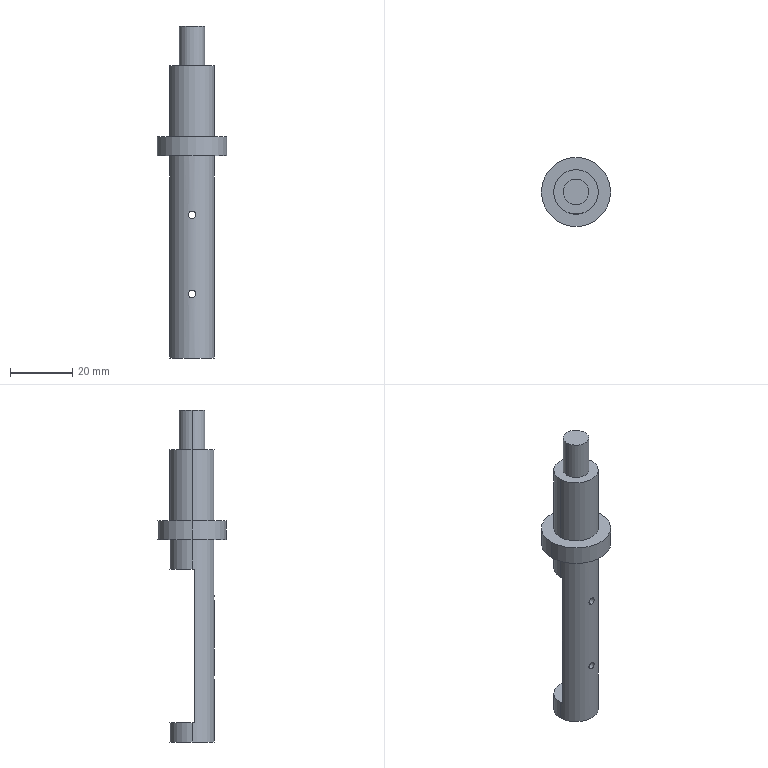Part | SolidWorks | features ICE 6, HoleWzd 2, Extrusion 1, RefAxis 1 | 1 solid | 25 faces | box 22.225 x 22.225 x 106.629 mm | volume 12564 mm3 | cylinder 13 | plane 8 | cone 4 | commonest cylinder face diameters 2.375 x4 14.275 x3 8.255 x2 14.3 x2 22.225 x2
STEP:
#1=CARTESIAN_POINT('',(0.,-0.06425,-2.435));
#2=VERTEX_POINT('',#1);
#3=CARTESIAN_POINT('',(0.,-0.06425,-2.341));
#4=VERTEX_POINT('',#3);
#5=CARTESIAN_POINT('',(0.,-0.06425,-2.388));
#6=DIRECTION('',(0.,1.,0.));
#7=DIRECTION('',(0.,0.,1.));
#8=AXIS2_PLACEMENT_3D('',#5,#6,#7);
#9=CIRCLE('',#8,0.04675);
#10=EDGE_CURVE('',#2,#4,#9,.T.);
#11=ORIENTED_EDGE('',*,*,#10,.F.);
#12=CARTESIAN_POINT('',(0.,-0.03,-2.469));
#13=VERTEX_POINT('',#12);
#14=CARTESIAN_POINT('',(0.,-0.03,-2.469));
#15=DIRECTION('',(0.,0.7071,-0.7071));
#16=VECTOR('',#15,39.37);
#17=LINE('',#14,#16);
#18=EDGE_CURVE('',#2,#13,#17,.T.);
#19=ORIENTED_EDGE('',*,*,#18,.T.);
#20=CARTESIAN_POINT('',(0.,-0.03,-2.307));
#21=VERTEX_POINT('',#20);
#22=CARTESIAN_POINT('',(0.,-0.03,-2.388));
#23=DIRECTION('',(0.,1.,0.));
#24=DIRECTION('',(0.,0.,1.));
#25=AXIS2_PLACEMENT_3D('',#22,#23,#24);
#26=CIRCLE('',#25,0.081);
#27=EDGE_CURVE('',#13,#21,#26,.T.);
#28=ORIENTED_EDGE('',*,*,#27,.T.);
#29=CARTESIAN_POINT('',(0.,-0.03,-2.307));
#30=DIRECTION('',(0.,0.7071,0.7071));
#31=VECTOR('',#30,39.37);
#32=LINE('',#29,#31);
#33=EDGE_CURVE('',#4,#21,#32,.T.);
#34=ORIENTED_EDGE('',*,*,#33,.F.);
#35=EDGE_LOOP('',(#11,#19,#28,#34));
#36=FACE_OUTER_BOUND('',#35,.T.);
#37=CARTESIAN_POINT('',(0.,-0.03,-2.388));
#38=DIRECTION('',(0.,1.,0.));
#39=DIRECTION('',(0.,0.,1.));
#40=AXIS2_PLACEMENT_3D('',#37,#38,#39);
#41=CONICAL_SURFACE('',#40,0.081,0.7854);
#42=ADVANCED_FACE('',(#36),#41,.F.);
#43=CARTESIAN_POINT('',(0.,-0.281,-2.341));
#44=VERTEX_POINT('',#43);
#45=CARTESIAN_POINT('',(0.,-0.281,-2.435));
#46=VERTEX_POINT('',#45);
#47=CARTESIAN_POINT('',(0.,-0.281,-2.341));
#48=CARTESIAN_POINT('',(-0.006189,-0.281,-2.341));
#49=CARTESIAN_POINT('',(-0.01226,-0.2808,-2.342));
#50=CARTESIAN_POINT('',(-0.02358,-0.2801,-2.347));
#51=CARTESIAN_POINT('',(-0.02876,-0.2796,-2.351));
#52=CARTESIAN_POINT('',(-0.03737,-0.2785,-2.359));
#53=CARTESIAN_POINT('',(-0.04085,-0.278,-2.364));
#54=CARTESIAN_POINT('',(-0.04552,-0.2773,-2.376));
#55=CARTESIAN_POINT('',(-0.04675,-0.2771,-2.382));
#56=CARTESIAN_POINT('',(-0.04675,-0.2771,-2.394));
#57=CARTESIAN_POINT('',(-0.04554,-0.2773,-2.4));
#58=CARTESIAN_POINT('',(-0.04084,-0.278,-2.412));
#59=CARTESIAN_POINT('',(-0.03741,-0.2785,-2.417));
#60=CARTESIAN_POINT('',(-0.0287,-0.2796,-2.425));
#61=CARTESIAN_POINT('',(-0.02356,-0.2801,-2.429));
#62=CARTESIAN_POINT('',(-0.01225,-0.2808,-2.434));
#63=CARTESIAN_POINT('',(-0.006108,-0.281,-2.435));
#64=CARTESIAN_POINT('',(0.,-0.281,-2.435));
#65=B_SPLINE_CURVE_WITH_KNOTS('',3,(#47,#48,#49,#50,#51,#52,#53,#54,#55,#56,#57,#58,#59,#60,#61,#62,#63,#64),.UNSPECIFIED.,.F.,.F.,(4,2,2,2,2,2,2,2,4),(0.,0.0004649,0.0009297,0.001395,0.001859,0.002324,0.002789,0.003254,0.003719),.UNSPECIFIED.);
#66=EDGE_CURVE('',#44,#46,#65,.T.);
#67=ORIENTED_EDGE('',*,*,#66,.T.);
#68=CARTESIAN_POINT('',(0.,-0.03,-2.435));
#69=DIRECTION('',(0.,1.,0.));
#70=VECTOR('',#69,39.37);
#71=LINE('',#68,#70);
#72=EDGE_CURVE('',#46,#2,#71,.T.);
#73=ORIENTED_EDGE('',*,*,#72,.T.);
#74=ORIENTED_EDGE('',*,*,#10,.T.);
#75=CARTESIAN_POINT('',(0.,-0.03,-2.341));
#76=DIRECTION('',(0.,1.,0.));
#77=VECTOR('',#76,39.37);
#78=LINE('',#75,#77);
#79=EDGE_CURVE('',#44,#4,#78,.T.);
#80=ORIENTED_EDGE('',*,*,#79,.F.);
#81=EDGE_LOOP('',(#67,#73,#74,#80));
#82=FACE_OUTER_BOUND('',#81,.T.);
#83=CARTESIAN_POINT('',(0.,-0.03,-2.388));
#84=DIRECTION('',(0.,1.,0.));
#85=DIRECTION('',(0.,0.,1.));
#86=AXIS2_PLACEMENT_3D('',#83,#84,#85);
#87=CYLINDRICAL_SURFACE('',#86,0.04675);
#88=ADVANCED_FACE('',(#82),#87,.F.);
#89=CARTESIAN_POINT('',(0.,-0.06425,-3.435));
#90=VERTEX_POINT('',#89);
#91=CARTESIAN_POINT('',(0.,-0.06425,-3.341));
#92=VERTEX_POINT('',#91);
#93=CARTESIAN_POINT('',(0.,-0.06425,-3.388));
#94=DIRECTION('',(0.,1.,0.));
#95=DIRECTION('',(0.,0.,1.));
#96=AXIS2_PLACEMENT_3D('',#93,#94,#95);
#97=CIRCLE('',#96,0.04675);
#98=EDGE_CURVE('',#90,#92,#97,.T.);
#99=ORIENTED_EDGE('',*,*,#98,.F.);
#100=CARTESIAN_POINT('',(0.,-0.03,-3.469));
#101=VERTEX_POINT('',#100);
#102=CARTESIAN_POINT('',(0.,-0.03,-3.469));
#103=DIRECTION('',(0.,0.7071,-0.7071));
#104=VECTOR('',#103,39.37);
#105=LINE('',#102,#104);
#106=EDGE_CURVE('',#90,#101,#105,.T.);
#107=ORIENTED_EDGE('',*,*,#106,.T.);
#108=CARTESIAN_POINT('',(0.,-0.03,-3.307));
#109=VERTEX_POINT('',#108);
#110=CARTESIAN_POINT('',(0.,-0.03,-3.388));
#111=DIRECTION('',(0.,1.,0.));
#112=DIRECTION('',(0.,0.,1.));
#113=AXIS2_PLACEMENT_3D('',#110,#111,#112);
#114=CIRCLE('',#113,0.081);
#115=EDGE_CURVE('',#101,#109,#114,.T.);
#116=ORIENTED_EDGE('',*,*,#115,.T.);
#117=CARTESIAN_POINT('',(0.,-0.03,-3.307));
#118=DIRECTION('',(0.,0.7071,0.7071));
#119=VECTOR('',#118,39.37);
#120=LINE('',#117,#119);
#121=EDGE_CURVE('',#92,#109,#120,.T.);
#122=ORIENTED_EDGE('',*,*,#121,.F.);
#123=EDGE_LOOP('',(#99,#107,#116,#122));
#124=FACE_OUTER_BOUND('',#123,.T.);
#125=CARTESIAN_POINT('',(0.,-0.03,-3.388));
#126=DIRECTION('',(0.,1.,0.));
#127=DIRECTION('',(0.,0.,1.));
#128=AXIS2_PLACEMENT_3D('',#125,#126,#127);
#129=CONICAL_SURFACE('',#128,0.081,0.7854);
#130=ADVANCED_FACE('',(#124),#129,.F.);
#131=CARTESIAN_POINT('',(0.,-0.281,-3.341));
#132=VERTEX_POINT('',#131);
#133=CARTESIAN_POINT('',(0.,-0.281,-3.435));
#134=VERTEX_POINT('',#133);
#135=CARTESIAN_POINT('',(0.,-0.281,-3.341));
#136=CARTESIAN_POINT('',(-0.006189,-0.281,-3.341));
#137=CARTESIAN_POINT('',(-0.01226,-0.2808,-3.342));
#138=CARTESIAN_POINT('',(-0.02358,-0.2801,-3.347));
#139=CARTESIAN_POINT('',(-0.02876,-0.2796,-3.351));
#140=CARTESIAN_POINT('',(-0.03737,-0.2785,-3.359));
#141=CARTESIAN_POINT('',(-0.04085,-0.278,-3.364));
#142=CARTESIAN_POINT('',(-0.04552,-0.2773,-3.376));
#143=CARTESIAN_POINT('',(-0.04675,-0.2771,-3.382));
#144=CARTESIAN_POINT('',(-0.04675,-0.2771,-3.394));
#145=CARTESIAN_POINT('',(-0.04554,-0.2773,-3.4));
#146=CARTESIAN_POINT('',(-0.04084,-0.278,-3.412));
#147=CARTESIAN_POINT('',(-0.03741,-0.2785,-3.417));
#148=CARTESIAN_POINT('',(-0.0287,-0.2796,-3.425));
#149=CARTESIAN_POINT('',(-0.02356,-0.2801,-3.429));
#150=CARTESIAN_POINT('',(-0.01225,-0.2808,-3.434));
#151=CARTESIAN_POINT('',(-0.006108,-0.281,-3.435));
#152=CARTESIAN_POINT('',(0.,-0.281,-3.435));
#153=B_SPLINE_CURVE_WITH_KNOTS('',3,(#135,#136,#137,#138,#139,#140,#141,#142,#143,#144,#145,#146,#147,#148,#149,#150,#151,#152),.UNSPECIFIED.,.F.,.F.,(4,2,2,2,2,2,2,2,4),(0.,0.0004649,0.0009297,0.001395,0.001859,0.002324,0.002789,0.003254,0.003719),.UNSPECIFIED.);
#154=EDGE_CURVE('',#132,#134,#153,.T.);
#155=ORIENTED_EDGE('',*,*,#154,.T.);
#156=CARTESIAN_POINT('',(0.,-0.03,-3.435));
#157=DIRECTION('',(0.,1.,0.));
#158=VECTOR('',#157,39.37);
#159=LINE('',#156,#158);
#160=EDGE_CURVE('',#134,#90,#159,.T.);
#161=ORIENTED_EDGE('',*,*,#160,.T.);
#162=ORIENTED_EDGE('',*,*,#98,.T.);
#163=CARTESIAN_POINT('',(0.,-0.03,-3.341));
#164=DIRECTION('',(0.,1.,0.));
#165=VECTOR('',#164,39.37);
#166=LINE('',#163,#165);
#167=EDGE_CURVE('',#132,#92,#166,.T.);
#168=ORIENTED_EDGE('',*,*,#167,.F.);
#169=EDGE_LOOP('',(#155,#161,#162,#168));
#170=FACE_OUTER_BOUND('',#169,.T.);
#171=CARTESIAN_POINT('',(0.,-0.03,-3.388));
#172=DIRECTION('',(0.,1.,0.));
#173=DIRECTION('',(0.,0.,1.));
#174=AXIS2_PLACEMENT_3D('',#171,#172,#173);
#175=CYLINDRICAL_SURFACE('',#174,0.04675);
#176=ADVANCED_FACE('',(#170),#175,.F.);
#177=CARTESIAN_POINT('',(-0.1625,0.,-0.5));
#178=VERTEX_POINT('',#177);
#179=CARTESIAN_POINT('',(0.1625,0.,-0.5));
#180=VERTEX_POINT('',#179);
#181=CARTESIAN_POINT('',(0.,0.,-0.5));
#182=DIRECTION('',(0.,0.,-1.));
#183=DIRECTION('',(1.,0.,0.));
#184=AXIS2_PLACEMENT_3D('',#181,#182,#183);
#185=CIRCLE('',#184,0.1625);
#186=EDGE_CURVE('',#178,#180,#185,.T.);
#187=ORIENTED_EDGE('',*,*,#186,.F.);
#188=CARTESIAN_POINT('',(-0.1625,0.,0.));
#189=VERTEX_POINT('',#188);
#190=CARTESIAN_POINT('',(-0.1625,0.,-1.75));
#191=DIRECTION('',(0.,0.,1.));
#192=VECTOR('',#191,39.37);
#193=LINE('',#190,#192);
#194=EDGE_CURVE('',#178,#189,#193,.T.);
#195=ORIENTED_EDGE('',*,*,#194,.T.);
#196=CARTESIAN_POINT('',(0.1625,0.,0.));
#197=VERTEX_POINT('',#196);
#198=CARTESIAN_POINT('',(0.,0.,0.));
#199=DIRECTION('',(0.,0.,1.));
#200=DIRECTION('',(1.,0.,0.));
#201=AXIS2_PLACEMENT_3D('',#198,#199,#200);
#202=CIRCLE('',#201,0.1625);
#203=EDGE_CURVE('',#197,#189,#202,.T.);
#204=ORIENTED_EDGE('',*,*,#203,.F.);
#205=CARTESIAN_POINT('',(0.1625,0.,-1.75));
#206=DIRECTION('',(0.,0.,1.));
#207=VECTOR('',#206,39.37);
#208=LINE('',#205,#207);
#209=EDGE_CURVE('',#180,#197,#208,.T.);
#210=ORIENTED_EDGE('',*,*,#209,.F.);
#211=EDGE_LOOP('',(#187,#195,#204,#210));
#212=FACE_OUTER_BOUND('',#211,.T.);
#213=CARTESIAN_POINT('',(0.,0.,-1.75));
#214=DIRECTION('',(0.,0.,1.));
#215=DIRECTION('',(1.,0.,0.));
#216=AXIS2_PLACEMENT_3D('',#213,#214,#215);
#217=CYLINDRICAL_SURFACE('',#216,0.1625);
#218=ADVANCED_FACE('',(#212),#217,.T.);
#219=CARTESIAN_POINT('',(-0.281,0.,-1.638));
#220=VERTEX_POINT('',#219);
#221=CARTESIAN_POINT('',(0.281,0.,-1.638));
#222=VERTEX_POINT('',#221);
#223=CARTESIAN_POINT('',(0.,0.,-1.638));
#224=DIRECTION('',(0.,0.,-1.));
#225=DIRECTION('',(1.,0.,0.));
#226=AXIS2_PLACEMENT_3D('',#223,#224,#225);
#227=CIRCLE('',#226,0.281);
#228=EDGE_CURVE('',#220,#222,#227,.T.);
#229=ORIENTED_EDGE('',*,*,#228,.T.);
#230=CARTESIAN_POINT('',(0.281,0.,-2.013));
#231=VERTEX_POINT('',#230);
#232=CARTESIAN_POINT('',(0.281,0.,-0.8432));
#233=DIRECTION('',(0.,0.,-1.));
#234=VECTOR('',#233,39.37);
#235=LINE('',#232,#234);
#236=EDGE_CURVE('',#222,#231,#235,.T.);
#237=ORIENTED_EDGE('',*,*,#236,.T.);
#238=CARTESIAN_POINT('',(-0.281,0.,-2.013));
#239=VERTEX_POINT('',#238);
#240=CARTESIAN_POINT('',(0.,0.,-2.013));
#241=DIRECTION('',(0.,0.,-1.));
#242=DIRECTION('',(-1.,0.,0.));
#243=AXIS2_PLACEMENT_3D('',#240,#241,#242);
#244=CIRCLE('',#243,0.281);
#245=EDGE_CURVE('',#239,#231,#244,.T.);
#246=ORIENTED_EDGE('',*,*,#245,.F.);
#247=CARTESIAN_POINT('',(-0.281,0.,-0.8432));
#248=DIRECTION('',(0.,0.,-1.));
#249=VECTOR('',#248,39.37);
#250=LINE('',#247,#249);
#251=EDGE_CURVE('',#220,#239,#250,.T.);
#252=ORIENTED_EDGE('',*,*,#251,.F.);
#253=EDGE_LOOP('',(#229,#237,#246,#252));
#254=FACE_OUTER_BOUND('',#253,.T.);
#255=CARTESIAN_POINT('',(0.,0.,-0.8432));
#256=DIRECTION('',(0.,0.,-1.));
#257=DIRECTION('',(-1.,0.,0.));
#258=AXIS2_PLACEMENT_3D('',#255,#256,#257);
#259=CYLINDRICAL_SURFACE('',#258,0.281);
#260=ADVANCED_FACE('',(#254),#259,.T.);
#261=CARTESIAN_POINT('',(-0.281,0.,-3.957));
#262=VERTEX_POINT('',#261);
#263=CARTESIAN_POINT('',(0.281,0.,-3.957));
#264=VERTEX_POINT('',#263);
#265=CARTESIAN_POINT('',(0.,0.,-3.957));
#266=DIRECTION('',(0.,0.,-1.));
#267=DIRECTION('',(-1.,0.,0.));
#268=AXIS2_PLACEMENT_3D('',#265,#266,#267);
#269=CIRCLE('',#268,0.281);
#270=EDGE_CURVE('',#262,#264,#269,.T.);
#271=ORIENTED_EDGE('',*,*,#270,.T.);
#272=CARTESIAN_POINT('',(0.281,0.,-4.198));
#273=VERTEX_POINT('',#272);
#274=CARTESIAN_POINT('',(0.281,0.,-0.8432));
#275=DIRECTION('',(0.,0.,-1.));
#276=VECTOR('',#275,39.37);
#277=LINE('',#274,#276);
#278=EDGE_CURVE('',#264,#273,#277,.T.);
#279=ORIENTED_EDGE('',*,*,#278,.T.);
#280=CARTESIAN_POINT('',(-0.281,0.,-4.198));
#281=VERTEX_POINT('',#280);
#282=CARTESIAN_POINT('',(0.,0.,-4.198));
#283=DIRECTION('',(0.,0.,-1.));
#284=DIRECTION('',(-1.,0.,0.));
#285=AXIS2_PLACEMENT_3D('',#282,#283,#284);
#286=CIRCLE('',#285,0.281);
#287=EDGE_CURVE('',#281,#273,#286,.T.);
#288=ORIENTED_EDGE('',*,*,#287,.F.);
#289=CARTESIAN_POINT('',(-0.281,0.,-0.8432));
#290=DIRECTION('',(0.,0.,-1.));
#291=VECTOR('',#290,39.37);
#292=LINE('',#289,#291);
#293=EDGE_CURVE('',#262,#281,#292,.T.);
#294=ORIENTED_EDGE('',*,*,#293,.F.);
#295=EDGE_LOOP('',(#271,#279,#288,#294));
#296=FACE_OUTER_BOUND('',#295,.T.);
#297=CARTESIAN_POINT('',(0.,0.,-0.8432));
#298=DIRECTION('',(0.,0.,-1.));
#299=DIRECTION('',(-1.,0.,0.));
#300=AXIS2_PLACEMENT_3D('',#297,#298,#299);
#301=CYLINDRICAL_SURFACE('',#300,0.281);
#302=ADVANCED_FACE('',(#296),#301,.T.);
#303=CARTESIAN_POINT('',(0.4375,0.,-1.638));
#304=VERTEX_POINT('',#303);
#305=CARTESIAN_POINT('',(-0.4375,0.,-1.638));
#306=VERTEX_POINT('',#305);
#307=CARTESIAN_POINT('',(0.,0.,-1.638));
#308=DIRECTION('',(0.,0.,1.));
#309=DIRECTION('',(1.,0.,0.));
#310=AXIS2_PLACEMENT_3D('',#307,#308,#309);
#311=CIRCLE('',#310,0.4375);
#312=EDGE_CURVE('',#304,#306,#311,.T.);
#313=ORIENTED_EDGE('',*,*,#312,.T.);
#314=CARTESIAN_POINT('',(-0.4375,0.,-1.398));
#315=VERTEX_POINT('',#314);
#316=CARTESIAN_POINT('',(-0.4375,0.,-1.638));
#317=DIRECTION('',(0.,0.,1.));
#318=VECTOR('',#317,39.37);
#319=LINE('',#316,#318);
#320=EDGE_CURVE('',#306,#315,#319,.T.);
#321=ORIENTED_EDGE('',*,*,#320,.T.);
#322=CARTESIAN_POINT('',(0.4375,0.,-1.398));
#323=VERTEX_POINT('',#322);
#324=CARTESIAN_POINT('',(0.,0.,-1.398));
#325=DIRECTION('',(0.,0.,1.));
#326=DIRECTION('',(1.,0.,0.));
#327=AXIS2_PLACEMENT_3D('',#324,#325,#326);
#328=CIRCLE('',#327,0.4375);
#329=EDGE_CURVE('',#323,#315,#328,.T.);
#330=ORIENTED_EDGE('',*,*,#329,.F.);
#331=CARTESIAN_POINT('',(0.4375,0.,-1.638));
#332=DIRECTION('',(0.,0.,1.));
#333=VECTOR('',#332,39.37);
#334=LINE('',#331,#333);
#335=EDGE_CURVE('',#304,#323,#334,.T.);
#336=ORIENTED_EDGE('',*,*,#335,.F.);
#337=EDGE_LOOP('',(#313,#321,#330,#336));
#338=FACE_OUTER_BOUND('',#337,.T.);
#339=CARTESIAN_POINT('',(0.,0.,-1.638));
#340=DIRECTION('',(0.,0.,1.));
#341=DIRECTION('',(1.,0.,0.));
#342=AXIS2_PLACEMENT_3D('',#339,#340,#341);
#343=CYLINDRICAL_SURFACE('',#342,0.4375);
#344=ADVANCED_FACE('',(#338),#343,.T.);
#345=CARTESIAN_POINT('',(-0.2815,0.,-1.398));
#346=VERTEX_POINT('',#345);
#347=CARTESIAN_POINT('',(0.2815,0.,-1.398));
#348=VERTEX_POINT('',#347);
#349=CARTESIAN_POINT('',(0.,0.,-1.398));
#350=DIRECTION('',(0.,0.,-1.));
#351=DIRECTION('',(1.,0.,0.));
#352=AXIS2_PLACEMENT_3D('',#349,#350,#351);
#353=CIRCLE('',#352,0.2815);
#354=EDGE_CURVE('',#346,#348,#353,.T.);
#355=ORIENTED_EDGE('',*,*,#354,.F.);
#356=CARTESIAN_POINT('',(-0.2815,0.,-0.5));
#357=VERTEX_POINT('',#356);
#358=CARTESIAN_POINT('',(-0.2815,0.,-4.198));
#359=DIRECTION('',(0.,0.,1.));
#360=VECTOR('',#359,39.37);
#361=LINE('',#358,#360);
#362=EDGE_CURVE('',#346,#357,#361,.T.);
#363=ORIENTED_EDGE('',*,*,#362,.T.);
#364=CARTESIAN_POINT('',(0.2815,0.,-0.5));
#365=VERTEX_POINT('',#364);
#366=CARTESIAN_POINT('',(0.,0.,-0.5));
#367=DIRECTION('',(0.,0.,-1.));
#368=DIRECTION('',(1.,0.,0.));
#369=AXIS2_PLACEMENT_3D('',#366,#367,#368);
#370=CIRCLE('',#369,0.2815);
#371=EDGE_CURVE('',#357,#365,#370,.T.);
#372=ORIENTED_EDGE('',*,*,#371,.T.);
#373=CARTESIAN_POINT('',(0.2815,0.,-4.198));
#374=DIRECTION('',(0.,0.,1.));
#375=VECTOR('',#374,39.37);
#376=LINE('',#373,#375);
#377=EDGE_CURVE('',#348,#365,#376,.T.);
#378=ORIENTED_EDGE('',*,*,#377,.F.);
#379=EDGE_LOOP('',(#355,#363,#372,#378));
#380=FACE_OUTER_BOUND('',#379,.T.);
#381=CARTESIAN_POINT('',(0.,0.,-4.198));
#382=DIRECTION('',(0.,0.,1.));
#383=DIRECTION('',(1.,0.,0.));
#384=AXIS2_PLACEMENT_3D('',#381,#382,#383);
#385=CYLINDRICAL_SURFACE('',#384,0.2815);
#386=ADVANCED_FACE('',(#380),#385,.T.);
#387=ORIENTED_EDGE('',*,*,#362,.F.);
#388=CARTESIAN_POINT('',(0.,0.,-1.398));
#389=DIRECTION('',(0.,0.,-1.));
#390=DIRECTION('',(1.,0.,0.));
#391=AXIS2_PLACEMENT_3D('',#388,#389,#390);
#392=CIRCLE('',#391,0.2815);
#393=EDGE_CURVE('',#348,#346,#392,.T.);
#394=ORIENTED_EDGE('',*,*,#393,.F.);
#395=ORIENTED_EDGE('',*,*,#377,.T.);
#396=CARTESIAN_POINT('',(0.,0.,-0.5));
#397=DIRECTION('',(0.,0.,-1.));
#398=DIRECTION('',(1.,0.,0.));
#399=AXIS2_PLACEMENT_3D('',#396,#397,#398);
#400=CIRCLE('',#399,0.2815);
#401=EDGE_CURVE('',#365,#357,#400,.T.);
#402=ORIENTED_EDGE('',*,*,#401,.T.);
#403=EDGE_LOOP('',(#387,#394,#395,#402));
#404=FACE_OUTER_BOUND('',#403,.T.);
#405=CARTESIAN_POINT('',(0.,0.,-4.198));
#406=DIRECTION('',(0.,0.,1.));
#407=DIRECTION('',(1.,0.,0.));
#408=AXIS2_PLACEMENT_3D('',#405,#406,#407);
#409=CYLINDRICAL_SURFACE('',#408,0.2815);
#410=ADVANCED_FACE('',(#404),#409,.T.);
#411=ORIENTED_EDGE('',*,*,#320,.F.);
#412=CARTESIAN_POINT('',(0.,0.,-1.638));
#413=DIRECTION('',(0.,0.,1.));
#414=DIRECTION('',(1.,0.,0.));
#415=AXIS2_PLACEMENT_3D('',#412,#413,#414);
#416=CIRCLE('',#415,0.4375);
#417=EDGE_CURVE('',#306,#304,#416,.T.);
#418=ORIENTED_EDGE('',*,*,#417,.T.);
#419=ORIENTED_EDGE('',*,*,#335,.T.);
#420=CARTESIAN_POINT('',(0.,0.,-1.398));
#421=DIRECTION('',(0.,0.,1.));
#422=DIRECTION('',(1.,0.,0.));
#423=AXIS2_PLACEMENT_3D('',#420,#421,#422);
#424=CIRCLE('',#423,0.4375);
#425=EDGE_CURVE('',#315,#323,#424,.T.);
#426=ORIENTED_EDGE('',*,*,#425,.F.);
#427=EDGE_LOOP('',(#411,#418,#419,#426));
#428=FACE_OUTER_BOUND('',#427,.T.);
#429=CARTESIAN_POINT('',(0.,0.,-1.638));
#430=DIRECTION('',(0.,0.,1.));
#431=DIRECTION('',(1.,0.,0.));
#432=AXIS2_PLACEMENT_3D('',#429,#430,#431);
#433=CYLINDRICAL_SURFACE('',#432,0.4375);
#434=ADVANCED_FACE('',(#428),#433,.T.);
#435=ORIENTED_EDGE('',*,*,#312,.F.);
#436=ORIENTED_EDGE('',*,*,#417,.F.);
#437=EDGE_LOOP('',(#435,#436));
#438=FACE_OUTER_BOUND('',#437,.T.);
#439=ORIENTED_EDGE('',*,*,#228,.F.);
#440=CARTESIAN_POINT('',(0.,0.,-1.638));
#441=DIRECTION('',(0.,0.,-1.));
#442=DIRECTION('',(1.,0.,0.));
#443=AXIS2_PLACEMENT_3D('',#440,#441,#442);
#444=CIRCLE('',#443,0.281);
#445=EDGE_CURVE('',#222,#220,#444,.T.);
#446=ORIENTED_EDGE('',*,*,#445,.F.);
#447=EDGE_LOOP('',(#439,#446));
#448=FACE_BOUND('',#447,.T.);
#449=CARTESIAN_POINT('',(0.,0.,-1.638));
#450=DIRECTION('',(0.,0.,1.));
#451=DIRECTION('',(1.,0.,0.));
#452=AXIS2_PLACEMENT_3D('',#449,#450,#451);
#453=PLANE('',#452);
#454=ADVANCED_FACE('',(#438,#448),#453,.F.);
#455=ORIENTED_EDGE('',*,*,#393,.T.);
#456=ORIENTED_EDGE('',*,*,#354,.T.);
#457=EDGE_LOOP('',(#455,#456));
#458=FACE_BOUND('',#457,.T.);
#459=ORIENTED_EDGE('',*,*,#329,.T.);
#460=ORIENTED_EDGE('',*,*,#425,.T.);
#461=EDGE_LOOP('',(#459,#460));
#462=FACE_OUTER_BOUND('',#461,.T.);
#463=CARTESIAN_POINT('',(0.,0.,-1.398));
#464=DIRECTION('',(0.,0.,1.));
#465=DIRECTION('',(1.,0.,0.));
#466=AXIS2_PLACEMENT_3D('',#463,#464,#465);
#467=PLANE('',#466);
#468=ADVANCED_FACE('',(#458,#462),#467,.T.);
#469=ORIENTED_EDGE('',*,*,#236,.F.);
#470=ORIENTED_EDGE('',*,*,#445,.T.);
#471=ORIENTED_EDGE('',*,*,#251,.T.);
#472=CARTESIAN_POINT('',(-0.2794,-0.03,-2.013));
#473=VERTEX_POINT('',#472);
#474=CARTESIAN_POINT('',(0.,0.,-2.013));
#475=DIRECTION('',(0.,0.,-1.));
#476=DIRECTION('',(-1.,0.,0.));
#477=AXIS2_PLACEMENT_3D('',#474,#475,#476);
#478=CIRCLE('',#477,0.281);
#479=EDGE_CURVE('',#473,#239,#478,.T.);
#480=ORIENTED_EDGE('',*,*,#479,.F.);
#481=CARTESIAN_POINT('',(-0.2794,-0.03,-3.957));
#482=VERTEX_POINT('',#481);
#483=CARTESIAN_POINT('',(-0.2794,-0.03,-3.957));
#484=DIRECTION('',(0.,0.,1.));
#485=VECTOR('',#484,39.37);
#486=LINE('',#483,#485);
#487=EDGE_CURVE('',#482,#473,#486,.T.);
#488=ORIENTED_EDGE('',*,*,#487,.F.);
#489=CARTESIAN_POINT('',(0.,0.,-3.957));
#490=DIRECTION('',(0.,0.,-1.));
#491=DIRECTION('',(-1.,0.,0.));
#492=AXIS2_PLACEMENT_3D('',#489,#490,#491);
#493=CIRCLE('',#492,0.281);
#494=EDGE_CURVE('',#482,#262,#493,.T.);
#495=ORIENTED_EDGE('',*,*,#494,.T.);
#496=ORIENTED_EDGE('',*,*,#293,.T.);
#497=CARTESIAN_POINT('',(0.,0.,-4.198));
#498=DIRECTION('',(0.,0.,-1.));
#499=DIRECTION('',(-1.,0.,0.));
#500=AXIS2_PLACEMENT_3D('',#497,#498,#499);
#501=CIRCLE('',#500,0.281);
#502=EDGE_CURVE('',#273,#281,#501,.T.);
#503=ORIENTED_EDGE('',*,*,#502,.F.);
#504=ORIENTED_EDGE('',*,*,#278,.F.);
#505=CARTESIAN_POINT('',(0.2794,-0.03,-3.957));
#506=VERTEX_POINT('',#505);
#507=CARTESIAN_POINT('',(0.,0.,-3.957));
#508=DIRECTION('',(0.,0.,-1.));
#509=DIRECTION('',(-1.,0.,0.));
#510=AXIS2_PLACEMENT_3D('',#507,#508,#509);
#511=CIRCLE('',#510,0.281);
#512=EDGE_CURVE('',#264,#506,#511,.T.);
#513=ORIENTED_EDGE('',*,*,#512,.T.);
#514=CARTESIAN_POINT('',(0.2794,-0.03,-2.013));
#515=VERTEX_POINT('',#514);
#516=CARTESIAN_POINT('',(0.2794,-0.03,-3.957));
#517=DIRECTION('',(0.,0.,1.));
#518=VECTOR('',#517,39.37);
#519=LINE('',#516,#518);
#520=EDGE_CURVE('',#506,#515,#519,.T.);
#521=ORIENTED_EDGE('',*,*,#520,.T.);
#522=CARTESIAN_POINT('',(0.,0.,-2.013));
#523=DIRECTION('',(0.,0.,-1.));
#524=DIRECTION('',(-1.,0.,0.));
#525=AXIS2_PLACEMENT_3D('',#522,#523,#524);
#526=CIRCLE('',#525,0.281);
#527=EDGE_CURVE('',#231,#515,#526,.T.);
#528=ORIENTED_EDGE('',*,*,#527,.F.);
#529=EDGE_LOOP('',(#469,#470,#471,#480,#488,#495,#496,#503,#504,#513,#521,#528));
#530=FACE_OUTER_BOUND('',#529,.T.);
#531=ORIENTED_EDGE('',*,*,#66,.F.);
#532=CARTESIAN_POINT('',(0.,-0.281,-2.435));
#533=CARTESIAN_POINT('',(0.006106,-0.281,-2.435));
#534=CARTESIAN_POINT('',(0.01227,-0.2808,-2.434));
#535=CARTESIAN_POINT('',(0.02352,-0.2801,-2.429));
#536=CARTESIAN_POINT('',(0.02872,-0.2796,-2.425));
#537=CARTESIAN_POINT('',(0.03735,-0.2785,-2.417));
#538=CARTESIAN_POINT('',(0.04081,-0.278,-2.412));
#539=CARTESIAN_POINT('',(0.04552,-0.2773,-2.4));
#540=CARTESIAN_POINT('',(0.04675,-0.2771,-2.394));
#541=CARTESIAN_POINT('',(0.04675,-0.2771,-2.382));
#542=CARTESIAN_POINT('',(0.04553,-0.2773,-2.376));
#543=CARTESIAN_POINT('',(0.04085,-0.278,-2.364));
#544=CARTESIAN_POINT('',(0.03738,-0.2785,-2.359));
#545=CARTESIAN_POINT('',(0.02878,-0.2796,-2.351));
#546=CARTESIAN_POINT('',(0.02358,-0.2801,-2.347));
#547=CARTESIAN_POINT('',(0.01233,-0.2808,-2.342));
#548=CARTESIAN_POINT('',(0.006188,-0.281,-2.341));
#549=CARTESIAN_POINT('',(0.,-0.281,-2.341));
#550=B_SPLINE_CURVE_WITH_KNOTS('',3,(#532,#533,#534,#535,#536,#537,#538,#539,#540,#541,#542,#543,#544,#545,#546,#547,#548,#549),.UNSPECIFIED.,.F.,.F.,(4,2,2,2,2,2,2,2,4),(0.003719,0.004184,0.004648,0.005113,0.005578,0.006043,0.006508,0.006972,0.007437),.UNSPECIFIED.);
#551=EDGE_CURVE('',#46,#44,#550,.T.);
#552=ORIENTED_EDGE('',*,*,#551,.F.);
#553=EDGE_LOOP('',(#531,#552));
#554=FACE_BOUND('',#553,.T.);
#555=ORIENTED_EDGE('',*,*,#154,.F.);
#556=CARTESIAN_POINT('',(0.,-0.281,-3.435));
#557=CARTESIAN_POINT('',(0.006106,-0.281,-3.435));
#558=CARTESIAN_POINT('',(0.01227,-0.2808,-3.434));
#559=CARTESIAN_POINT('',(0.02352,-0.2801,-3.429));
#560=CARTESIAN_POINT('',(0.02872,-0.2796,-3.425));
#561=CARTESIAN_POINT('',(0.03735,-0.2785,-3.417));
#562=CARTESIAN_POINT('',(0.04081,-0.278,-3.412));
#563=CARTESIAN_POINT('',(0.04552,-0.2773,-3.4));
#564=CARTESIAN_POINT('',(0.04675,-0.2771,-3.394));
#565=CARTESIAN_POINT('',(0.04675,-0.2771,-3.382));
#566=CARTESIAN_POINT('',(0.04553,-0.2773,-3.376));
#567=CARTESIAN_POINT('',(0.04085,-0.278,-3.364));
#568=CARTESIAN_POINT('',(0.03738,-0.2785,-3.359));
#569=CARTESIAN_POINT('',(0.02878,-0.2796,-3.351));
#570=CARTESIAN_POINT('',(0.02358,-0.2801,-3.347));
#571=CARTESIAN_POINT('',(0.01233,-0.2808,-3.342));
#572=CARTESIAN_POINT('',(0.006188,-0.281,-3.341));
#573=CARTESIAN_POINT('',(0.,-0.281,-3.341));
#574=B_SPLINE_CURVE_WITH_KNOTS('',3,(#556,#557,#558,#559,#560,#561,#562,#563,#564,#565,#566,#567,#568,#569,#570,#571,#572,#573),.UNSPECIFIED.,.F.,.F.,(4,2,2,2,2,2,2,2,4),(0.003719,0.004184,0.004648,0.005113,0.005578,0.006043,0.006508,0.006972,0.007437),.UNSPECIFIED.);
#575=EDGE_CURVE('',#134,#132,#574,.T.);
#576=ORIENTED_EDGE('',*,*,#575,.F.);
#577=EDGE_LOOP('',(#555,#576));
#578=FACE_BOUND('',#577,.T.);
#579=CARTESIAN_POINT('',(0.,0.,-0.8432));
#580=DIRECTION('',(0.,0.,-1.));
#581=DIRECTION('',(-1.,0.,0.));
#582=AXIS2_PLACEMENT_3D('',#579,#580,#581);
#583=CYLINDRICAL_SURFACE('',#582,0.281);
#584=ADVANCED_FACE('',(#530,#554,#578),#583,.T.);
#585=ORIENTED_EDGE('',*,*,#287,.T.);
#586=ORIENTED_EDGE('',*,*,#502,.T.);
#587=EDGE_LOOP('',(#585,#586));
#588=FACE_OUTER_BOUND('',#587,.T.);
#589=CARTESIAN_POINT('',(0.,0.,-4.198));
#590=DIRECTION('',(0.,0.,1.));
#591=DIRECTION('',(1.,0.,0.));
#592=AXIS2_PLACEMENT_3D('',#589,#590,#591);
#593=PLANE('',#592);
#594=ADVANCED_FACE('',(#588),#593,.F.);
#595=CARTESIAN_POINT('',(0.,-0.03,-2.388));
#596=DIRECTION('',(0.,1.,0.));
#597=DIRECTION('',(0.,0.,1.));
#598=AXIS2_PLACEMENT_3D('',#595,#596,#597);
#599=CIRCLE('',#598,0.081);
#600=EDGE_CURVE('',#21,#13,#599,.T.);
#601=ORIENTED_EDGE('',*,*,#600,.F.);
#602=ORIENTED_EDGE('',*,*,#27,.F.);
#603=EDGE_LOOP('',(#601,#602));
#604=FACE_BOUND('',#603,.T.);
#605=CARTESIAN_POINT('',(0.,-0.03,-3.388));
#606=DIRECTION('',(0.,1.,0.));
#607=DIRECTION('',(0.,0.,1.));
#608=AXIS2_PLACEMENT_3D('',#605,#606,#607);
#609=CIRCLE('',#608,0.081);
#610=EDGE_CURVE('',#109,#101,#609,.T.);
#611=ORIENTED_EDGE('',*,*,#610,.F.);
#612=ORIENTED_EDGE('',*,*,#115,.F.);
#613=EDGE_LOOP('',(#611,#612));
#614=FACE_BOUND('',#613,.T.);
#615=CARTESIAN_POINT('',(0.2794,-0.03,-2.013));
#616=DIRECTION('',(-1.,0.,0.));
#617=VECTOR('',#616,39.37);
#618=LINE('',#615,#617);
#619=EDGE_CURVE('',#515,#473,#618,.T.);
#620=ORIENTED_EDGE('',*,*,#619,.F.);
#621=ORIENTED_EDGE('',*,*,#520,.F.);
#622=CARTESIAN_POINT('',(0.2794,-0.03,-3.957));
#623=DIRECTION('',(-1.,0.,0.));
#624=VECTOR('',#623,39.37);
#625=LINE('',#622,#624);
#626=EDGE_CURVE('',#506,#482,#625,.T.);
#627=ORIENTED_EDGE('',*,*,#626,.T.);
#628=ORIENTED_EDGE('',*,*,#487,.T.);
#629=EDGE_LOOP('',(#620,#621,#627,#628));
#630=FACE_OUTER_BOUND('',#629,.T.);
#631=CARTESIAN_POINT('',(0.2794,-0.03,-3.957));
#632=DIRECTION('',(0.,1.,0.));
#633=DIRECTION('',(0.,0.,1.));
#634=AXIS2_PLACEMENT_3D('',#631,#632,#633);
#635=PLANE('',#634);
#636=ADVANCED_FACE('',(#604,#614,#630),#635,.T.);
#637=ORIENTED_EDGE('',*,*,#494,.F.);
#638=ORIENTED_EDGE('',*,*,#626,.F.);
#639=ORIENTED_EDGE('',*,*,#512,.F.);
#640=ORIENTED_EDGE('',*,*,#270,.F.);
#641=EDGE_LOOP('',(#637,#638,#639,#640));
#642=FACE_OUTER_BOUND('',#641,.T.);
#643=CARTESIAN_POINT('',(0.,0.,-3.957));
#644=DIRECTION('',(0.,0.,-1.));
#645=DIRECTION('',(-1.,0.,0.));
#646=AXIS2_PLACEMENT_3D('',#643,#644,#645);
#647=PLANE('',#646);
#648=ADVANCED_FACE('',(#642),#647,.F.);
#649=ORIENTED_EDGE('',*,*,#479,.T.);
#650=ORIENTED_EDGE('',*,*,#245,.T.);
#651=ORIENTED_EDGE('',*,*,#527,.T.);
#652=ORIENTED_EDGE('',*,*,#619,.T.);
#653=EDGE_LOOP('',(#649,#650,#651,#652));
#654=FACE_OUTER_BOUND('',#653,.T.);
#655=CARTESIAN_POINT('',(0.,0.,-2.013));
#656=DIRECTION('',(0.,0.,-1.));
#657=DIRECTION('',(-1.,0.,0.));
#658=AXIS2_PLACEMENT_3D('',#655,#656,#657);
#659=PLANE('',#658);
#660=ADVANCED_FACE('',(#654),#659,.T.);
#661=ORIENTED_EDGE('',*,*,#194,.F.);
#662=CARTESIAN_POINT('',(0.,0.,-0.5));
#663=DIRECTION('',(0.,0.,-1.));
#664=DIRECTION('',(1.,0.,0.));
#665=AXIS2_PLACEMENT_3D('',#662,#663,#664);
#666=CIRCLE('',#665,0.1625);
#667=EDGE_CURVE('',#180,#178,#666,.T.);
#668=ORIENTED_EDGE('',*,*,#667,.F.);
#669=ORIENTED_EDGE('',*,*,#209,.T.);
#670=CARTESIAN_POINT('',(0.,0.,0.));
#671=DIRECTION('',(0.,0.,1.));
#672=DIRECTION('',(1.,0.,0.));
#673=AXIS2_PLACEMENT_3D('',#670,#671,#672);
#674=CIRCLE('',#673,0.1625);
#675=EDGE_CURVE('',#189,#197,#674,.T.);
#676=ORIENTED_EDGE('',*,*,#675,.F.);
#677=EDGE_LOOP('',(#661,#668,#669,#676));
#678=FACE_OUTER_BOUND('',#677,.T.);
#679=CARTESIAN_POINT('',(0.,0.,-1.75));
#680=DIRECTION('',(0.,0.,1.));
#681=DIRECTION('',(1.,0.,0.));
#682=AXIS2_PLACEMENT_3D('',#679,#680,#681);
#683=CYLINDRICAL_SURFACE('',#682,0.1625);
#684=ADVANCED_FACE('',(#678),#683,.T.);
#685=ORIENTED_EDGE('',*,*,#401,.F.);
#686=ORIENTED_EDGE('',*,*,#371,.F.);
#687=EDGE_LOOP('',(#685,#686));
#688=FACE_OUTER_BOUND('',#687,.T.);
#689=ORIENTED_EDGE('',*,*,#667,.T.);
#690=ORIENTED_EDGE('',*,*,#186,.T.);
#691=EDGE_LOOP('',(#689,#690));
#692=FACE_BOUND('',#691,.T.);
#693=CARTESIAN_POINT('',(0.,0.,-0.5));
#694=DIRECTION('',(0.,0.,1.));
#695=DIRECTION('',(1.,0.,0.));
#696=AXIS2_PLACEMENT_3D('',#693,#694,#695);
#697=PLANE('',#696);
#698=ADVANCED_FACE('',(#688,#692),#697,.T.);
#699=ORIENTED_EDGE('',*,*,#203,.T.);
#700=ORIENTED_EDGE('',*,*,#675,.T.);
#701=EDGE_LOOP('',(#699,#700));
#702=FACE_OUTER_BOUND('',#701,.T.);
#703=CARTESIAN_POINT('',(0.,0.,0.));
#704=DIRECTION('',(0.,0.,1.));
#705=DIRECTION('',(1.,0.,0.));
#706=AXIS2_PLACEMENT_3D('',#703,#704,#705);
#707=PLANE('',#706);
#708=ADVANCED_FACE('',(#702),#707,.T.);
#709=ORIENTED_EDGE('',*,*,#160,.F.);
#710=ORIENTED_EDGE('',*,*,#575,.T.);
#711=ORIENTED_EDGE('',*,*,#167,.T.);
#712=CARTESIAN_POINT('',(0.,-0.06425,-3.388));
#713=DIRECTION('',(0.,1.,0.));
#714=DIRECTION('',(0.,0.,1.));
#715=AXIS2_PLACEMENT_3D('',#712,#713,#714);
#716=CIRCLE('',#715,0.04675);
#717=EDGE_CURVE('',#92,#90,#716,.T.);
#718=ORIENTED_EDGE('',*,*,#717,.T.);
#719=EDGE_LOOP('',(#709,#710,#711,#718));
#720=FACE_OUTER_BOUND('',#719,.T.);
#721=CARTESIAN_POINT('',(0.,-0.03,-3.388));
#722=DIRECTION('',(0.,1.,0.));
#723=DIRECTION('',(0.,0.,1.));
#724=AXIS2_PLACEMENT_3D('',#721,#722,#723);
#725=CYLINDRICAL_SURFACE('',#724,0.04675);
#726=ADVANCED_FACE('',(#720),#725,.F.);
#727=ORIENTED_EDGE('',*,*,#106,.F.);
#728=ORIENTED_EDGE('',*,*,#717,.F.);
#729=ORIENTED_EDGE('',*,*,#121,.T.);
#730=ORIENTED_EDGE('',*,*,#610,.T.);
#731=EDGE_LOOP('',(#727,#728,#729,#730));
#732=FACE_OUTER_BOUND('',#731,.T.);
#733=CARTESIAN_POINT('',(0.,-0.03,-3.388));
#734=DIRECTION('',(0.,1.,0.));
#735=DIRECTION('',(0.,0.,1.));
#736=AXIS2_PLACEMENT_3D('',#733,#734,#735);
#737=CONICAL_SURFACE('',#736,0.081,0.7854);
#738=ADVANCED_FACE('',(#732),#737,.F.);
#739=ORIENTED_EDGE('',*,*,#72,.F.);
#740=ORIENTED_EDGE('',*,*,#551,.T.);
#741=ORIENTED_EDGE('',*,*,#79,.T.);
#742=CARTESIAN_POINT('',(0.,-0.06425,-2.388));
#743=DIRECTION('',(0.,1.,0.));
#744=DIRECTION('',(0.,0.,1.));
#745=AXIS2_PLACEMENT_3D('',#742,#743,#744);
#746=CIRCLE('',#745,0.04675);
#747=EDGE_CURVE('',#4,#2,#746,.T.);
#748=ORIENTED_EDGE('',*,*,#747,.T.);
#749=EDGE_LOOP('',(#739,#740,#741,#748));
#750=FACE_OUTER_BOUND('',#749,.T.);
#751=CARTESIAN_POINT('',(0.,-0.03,-2.388));
#752=DIRECTION('',(0.,1.,0.));
#753=DIRECTION('',(0.,0.,1.));
#754=AXIS2_PLACEMENT_3D('',#751,#752,#753);
#755=CYLINDRICAL_SURFACE('',#754,0.04675);
#756=ADVANCED_FACE('',(#750),#755,.F.);
#757=ORIENTED_EDGE('',*,*,#18,.F.);
#758=ORIENTED_EDGE('',*,*,#747,.F.);
#759=ORIENTED_EDGE('',*,*,#33,.T.);
#760=ORIENTED_EDGE('',*,*,#600,.T.);
#761=EDGE_LOOP('',(#757,#758,#759,#760));
#762=FACE_OUTER_BOUND('',#761,.T.);
#763=CARTESIAN_POINT('',(0.,-0.03,-2.388));
#764=DIRECTION('',(0.,1.,0.));
#765=DIRECTION('',(0.,0.,1.));
#766=AXIS2_PLACEMENT_3D('',#763,#764,#765);
#767=CONICAL_SURFACE('',#766,0.081,0.7854);
#768=ADVANCED_FACE('',(#762),#767,.F.);
#769=CLOSED_SHELL('',(#42,#88,#130,#176,#218,#260,#302,#344,#386,#410,#434,#454,#468,#584,#594,#636,#648,#660,#684,#698,#708,#726,#738,#756,#768));
#770=MANIFOLD_SOLID_BREP('',#769);
#771=CARTESIAN_POINT('',(0.,0.,0.));
#772=DIRECTION('',(0.,0.,1.));
#773=DIRECTION('',(1.,0.,0.));
#774=AXIS2_PLACEMENT_3D('',#771,#772,#773);
#775=(LENGTH_UNIT()NAMED_UNIT(*)SI_UNIT($,.METRE.));
#776=LENGTH_MEASURE_WITH_UNIT(LENGTH_MEASURE(0.0254),#775);
#777=DIMENSIONAL_EXPONENTS(1.,0.,0.,0.,0.,0.,0.);
#778=(CONVERSION_BASED_UNIT('INCH',#776)LENGTH_UNIT()NAMED_UNIT(#777));
#779=UNCERTAINTY_MEASURE_WITH_UNIT(LENGTH_MEASURE(0.00001),#778,'','');
#780=(NAMED_UNIT(*)PLANE_ANGLE_UNIT()SI_UNIT($,.RADIAN.));
#781=(NAMED_UNIT(*)SI_UNIT($,.STERADIAN.)SOLID_ANGLE_UNIT());
#782=(GEOMETRIC_REPRESENTATION_CONTEXT(3)GLOBAL_UNCERTAINTY_ASSIGNED_CONTEXT((#779))GLOBAL_UNIT_ASSIGNED_CONTEXT((#778,#780,#781))REPRESENTATION_CONTEXT('',''));
#783=ADVANCED_BREP_SHAPE_REPRESENTATION('',(#770,#774),#782);